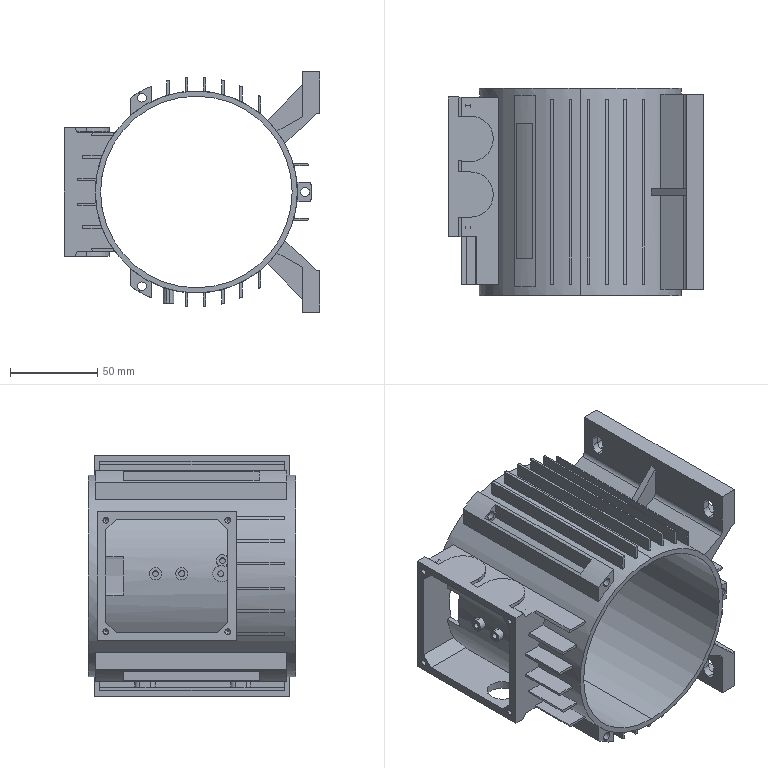Part | SolidWorks | features BaseBody 3 | 3 solids | 386 faces | box 147 x 119 x 138 mm | volume 264142 mm3 | plane 229 | cylinder 117 | cone 40 | commonest cylinder face diameters 3.3 x20 132 x19 5 x12 5.8 x12 8 x12 7 x7